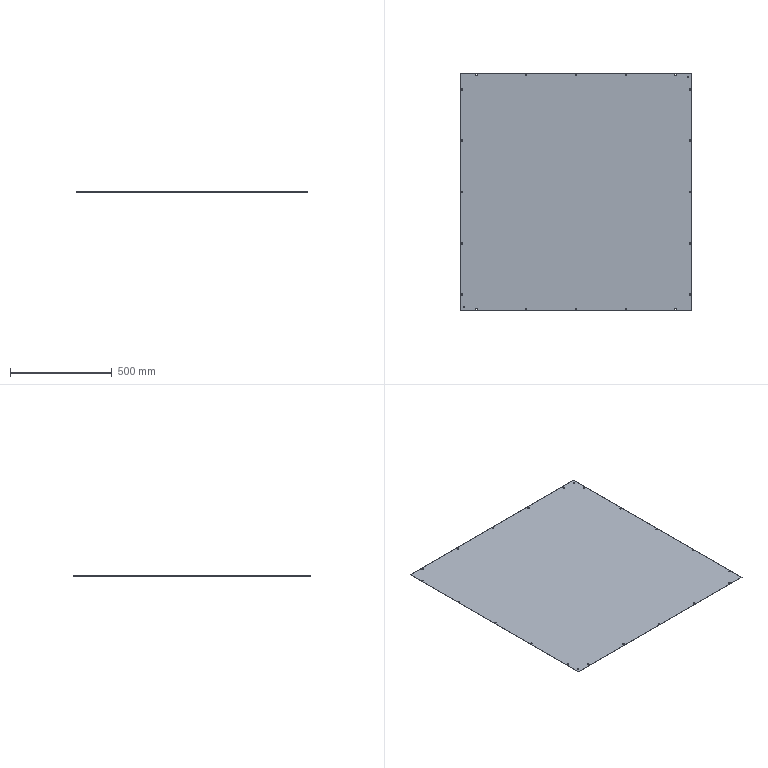Part | 1 solid | 100 faces | box 1140 x 1170 x 1 mm | volume 1332571 mm3 | cylinder 54 | plane 46 | commonest cylinder face diameters 7 x50 5 x4